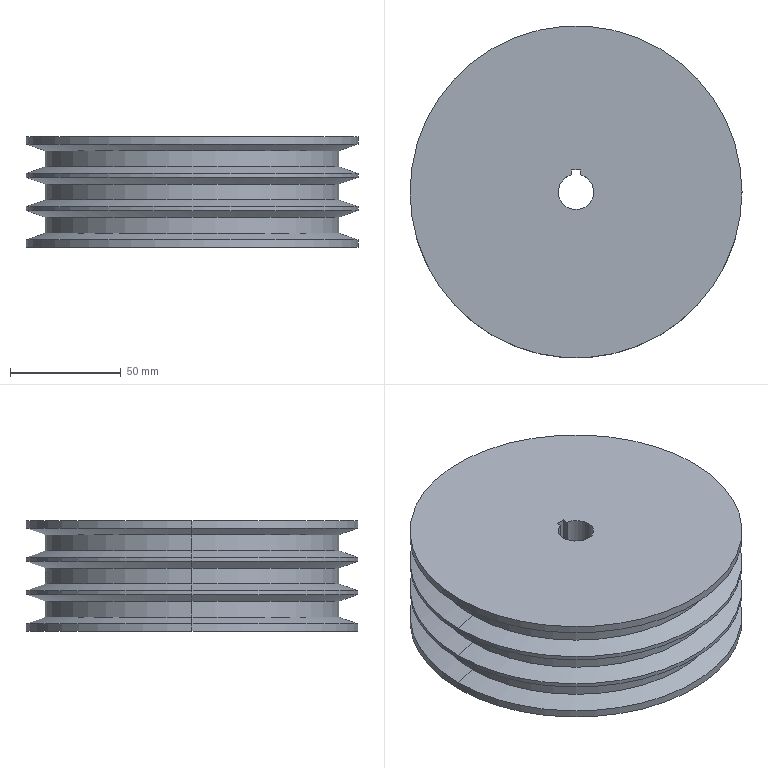Part | SolidWorks | features ICE 5, Extrusion 1, HoleWzd 1, RevCut 1 | 1 solid | 39 faces | box 150 x 150 x 50 mm | volume 752119 mm3 | cylinder 19 | cone 12 | plane 8 | commonest cylinder face diameters 150 x8 132.6 x6 16 x3 6.8 x2
STEP:
#1=CARTESIAN_POINT('',(0.,66.3,11.6));
#2=VERTEX_POINT('',#1);
#3=CARTESIAN_POINT('',(0.,66.3,18.4));
#4=VERTEX_POINT('',#3);
#5=CARTESIAN_POINT('',(0.,66.3,11.6));
#6=CARTESIAN_POINT('',(-0.2247,66.3,11.6));
#7=CARTESIAN_POINT('',(-0.4456,66.299,11.622));
#8=CARTESIAN_POINT('',(-0.8802,66.295,11.708));
#9=CARTESIAN_POINT('',(-1.096,66.291,11.774));
#10=CARTESIAN_POINT('',(-1.508,66.283,11.945));
#11=CARTESIAN_POINT('',(-1.703,66.278,12.049));
#12=CARTESIAN_POINT('',(-2.073,66.268,12.296));
#13=CARTESIAN_POINT('',(-2.248,66.262,12.439));
#14=CARTESIAN_POINT('',(-2.561,66.251,12.753));
#15=CARTESIAN_POINT('',(-2.702,66.245,12.924));
#16=CARTESIAN_POINT('',(-2.951,66.234,13.296));
#17=CARTESIAN_POINT('',(-3.056,66.23,13.494));
#18=CARTESIAN_POINT('',(-3.226,66.222,13.903));
#19=CARTESIAN_POINT('',(-3.291,66.218,14.117));
#20=CARTESIAN_POINT('',(-3.378,66.214,14.556));
#21=CARTESIAN_POINT('',(-3.4,66.213,14.777));
#22=CARTESIAN_POINT('',(-3.4,66.213,15.221));
#23=CARTESIAN_POINT('',(-3.378,66.214,15.446));
#24=CARTESIAN_POINT('',(-3.291,66.218,15.882));
#25=CARTESIAN_POINT('',(-3.227,66.221,16.094));
#26=CARTESIAN_POINT('',(-3.057,66.23,16.506));
#27=CARTESIAN_POINT('',(-2.95,66.234,16.705));
#28=CARTESIAN_POINT('',(-2.704,66.245,17.073));
#29=CARTESIAN_POINT('',(-2.563,66.251,17.245));
#30=CARTESIAN_POINT('',(-2.246,66.262,17.562));
#31=CARTESIAN_POINT('',(-2.074,66.268,17.703));
#32=CARTESIAN_POINT('',(-1.706,66.278,17.949));
#33=CARTESIAN_POINT('',(-1.507,66.283,18.056));
#34=CARTESIAN_POINT('',(-1.095,66.291,18.227));
#35=CARTESIAN_POINT('',(-0.883,66.294,18.291));
#36=CARTESIAN_POINT('',(-0.4473,66.299,18.378));
#37=CARTESIAN_POINT('',(-0.2219,66.3,18.4));
#38=CARTESIAN_POINT('',(0.,66.3,18.4));
#39=B_SPLINE_CURVE_WITH_KNOTS('',3,(#5,#6,#7,#8,#9,#10,#11,#12,#13,#14,#15,#16,#17,#18,#19,#20,#21,#22,#23,#24,#25,#26,#27,#28,#29,#30,#31,#32,#33,#34,#35,#36,#37,#38),.UNSPECIFIED.,.F.,.F.,(4,2,2,2,2,2,2,2,2,2,2,2,2,2,2,2,4),(0.,0.0006645,0.001329,0.001993,0.002658,0.003322,0.003987,0.004651,0.005316,0.00598,0.006645,0.007309,0.007974,0.008638,0.009303,0.009967,0.01063),.UNSPECIFIED.);
#40=EDGE_CURVE('',#2,#4,#39,.T.);
#41=ORIENTED_EDGE('',*,*,#40,.T.);
#42=CARTESIAN_POINT('',(0.,10.,18.4));
#43=VERTEX_POINT('',#42);
#44=CARTESIAN_POINT('',(0.,10.,18.4));
#45=DIRECTION('',(0.,-1.,0.));
#46=VECTOR('',#45,1000.);
#47=LINE('',#44,#46);
#48=EDGE_CURVE('',#4,#43,#47,.T.);
#49=ORIENTED_EDGE('',*,*,#48,.T.);
#50=CARTESIAN_POINT('',(-2.,10.,17.75));
#51=VERTEX_POINT('',#50);
#52=CARTESIAN_POINT('',(0.,10.,15.));
#53=DIRECTION('',(0.,-1.,0.));
#54=DIRECTION('',(0.,0.,-1.));
#55=AXIS2_PLACEMENT_3D('',#52,#53,#54);
#56=CIRCLE('',#55,3.4);
#57=EDGE_CURVE('',#43,#51,#56,.T.);
#58=ORIENTED_EDGE('',*,*,#57,.T.);
#59=CARTESIAN_POINT('',(-2.,10.,12.25));
#60=VERTEX_POINT('',#59);
#61=CARTESIAN_POINT('',(0.,10.,15.));
#62=DIRECTION('',(0.,-1.,0.));
#63=DIRECTION('',(0.,0.,-1.));
#64=AXIS2_PLACEMENT_3D('',#61,#62,#63);
#65=CIRCLE('',#64,3.4);
#66=EDGE_CURVE('',#51,#60,#65,.T.);
#67=ORIENTED_EDGE('',*,*,#66,.T.);
#68=CARTESIAN_POINT('',(0.,10.,11.6));
#69=VERTEX_POINT('',#68);
#70=CARTESIAN_POINT('',(0.,10.,15.));
#71=DIRECTION('',(0.,-1.,0.));
#72=DIRECTION('',(0.,0.,-1.));
#73=AXIS2_PLACEMENT_3D('',#70,#71,#72);
#74=CIRCLE('',#73,3.4);
#75=EDGE_CURVE('',#60,#69,#74,.T.);
#76=ORIENTED_EDGE('',*,*,#75,.T.);
#77=CARTESIAN_POINT('',(0.,10.,11.6));
#78=DIRECTION('',(0.,-1.,0.));
#79=VECTOR('',#78,1000.);
#80=LINE('',#77,#79);
#81=EDGE_CURVE('',#2,#69,#80,.T.);
#82=ORIENTED_EDGE('',*,*,#81,.F.);
#83=EDGE_LOOP('',(#41,#49,#58,#67,#76,#82));
#84=FACE_OUTER_BOUND('',#83,.T.);
#85=CARTESIAN_POINT('',(0.,10.,15.));
#86=DIRECTION('',(0.,-1.,0.));
#87=DIRECTION('',(0.,0.,-1.));
#88=AXIS2_PLACEMENT_3D('',#85,#86,#87);
#89=CYLINDRICAL_SURFACE('',#88,3.4);
#90=ADVANCED_FACE('',(#84),#89,.F.);
#91=CARTESIAN_POINT('',(66.3,0.,26.396));
#92=VERTEX_POINT('',#91);
#93=CARTESIAN_POINT('',(-66.3,0.,26.396));
#94=VERTEX_POINT('',#93);
#95=CARTESIAN_POINT('',(0.,0.,26.396));
#96=DIRECTION('',(0.,0.,1.));
#97=DIRECTION('',(1.,0.,0.));
#98=AXIS2_PLACEMENT_3D('',#95,#96,#97);
#99=CIRCLE('',#98,66.3);
#100=EDGE_CURVE('',#92,#94,#99,.T.);
#101=ORIENTED_EDGE('',*,*,#100,.F.);
#102=CARTESIAN_POINT('',(75.,0.,23.4));
#103=VERTEX_POINT('',#102);
#104=CARTESIAN_POINT('',(66.3,0.,26.396));
#105=DIRECTION('',(0.9455,0.,-0.3256));
#106=VECTOR('',#105,1000.);
#107=LINE('',#104,#106);
#108=EDGE_CURVE('',#92,#103,#107,.T.);
#109=ORIENTED_EDGE('',*,*,#108,.T.);
#110=CARTESIAN_POINT('',(-75.,0.,23.4));
#111=VERTEX_POINT('',#110);
#112=CARTESIAN_POINT('',(0.,0.,23.4));
#113=DIRECTION('',(0.,0.,1.));
#114=DIRECTION('',(1.,0.,0.));
#115=AXIS2_PLACEMENT_3D('',#112,#113,#114);
#116=CIRCLE('',#115,75.);
#117=EDGE_CURVE('',#103,#111,#116,.T.);
#118=ORIENTED_EDGE('',*,*,#117,.T.);
#119=CARTESIAN_POINT('',(-66.3,0.,26.396));
#120=DIRECTION('',(-0.9455,0.,-0.3256));
#121=VECTOR('',#120,1000.);
#122=LINE('',#119,#121);
#123=EDGE_CURVE('',#94,#111,#122,.T.);
#124=ORIENTED_EDGE('',*,*,#123,.F.);
#125=EDGE_LOOP('',(#101,#109,#118,#124));
#126=FACE_OUTER_BOUND('',#125,.T.);
#127=CARTESIAN_POINT('',(0.,0.,26.396));
#128=DIRECTION('',(0.,0.,-1.));
#129=DIRECTION('',(-1.,0.,0.));
#130=AXIS2_PLACEMENT_3D('',#127,#128,#129);
#131=CONICAL_SURFACE('',#130,66.3,1.239);
#132=ADVANCED_FACE('',(#126),#131,.T.);
#133=ORIENTED_EDGE('',*,*,#100,.T.);
#134=CARTESIAN_POINT('',(-66.3,0.,33.604));
#135=VERTEX_POINT('',#134);
#136=CARTESIAN_POINT('',(-66.3,0.,0.));
#137=DIRECTION('',(0.,0.,1.));
#138=VECTOR('',#137,1000.);
#139=LINE('',#136,#138);
#140=EDGE_CURVE('',#94,#135,#139,.T.);
#141=ORIENTED_EDGE('',*,*,#140,.T.);
#142=CARTESIAN_POINT('',(66.3,0.,33.604));
#143=VERTEX_POINT('',#142);
#144=CARTESIAN_POINT('',(0.,0.,33.604));
#145=DIRECTION('',(0.,0.,1.));
#146=DIRECTION('',(1.,0.,0.));
#147=AXIS2_PLACEMENT_3D('',#144,#145,#146);
#148=CIRCLE('',#147,66.3);
#149=EDGE_CURVE('',#143,#135,#148,.T.);
#150=ORIENTED_EDGE('',*,*,#149,.F.);
#151=CARTESIAN_POINT('',(66.3,0.,0.));
#152=DIRECTION('',(0.,0.,1.));
#153=VECTOR('',#152,1000.);
#154=LINE('',#151,#153);
#155=EDGE_CURVE('',#92,#143,#154,.T.);
#156=ORIENTED_EDGE('',*,*,#155,.F.);
#157=EDGE_LOOP('',(#133,#141,#150,#156));
#158=FACE_OUTER_BOUND('',#157,.T.);
#159=CARTESIAN_POINT('',(0.,0.,0.));
#160=DIRECTION('',(0.,0.,1.));
#161=DIRECTION('',(1.,0.,0.));
#162=AXIS2_PLACEMENT_3D('',#159,#160,#161);
#163=CYLINDRICAL_SURFACE('',#162,66.3);
#164=ADVANCED_FACE('',(#158),#163,.T.);
#165=ORIENTED_EDGE('',*,*,#149,.T.);
#166=CARTESIAN_POINT('',(-75.,0.,36.6));
#167=VERTEX_POINT('',#166);
#168=CARTESIAN_POINT('',(-75.,0.,36.6));
#169=DIRECTION('',(-0.9455,0.,0.3256));
#170=VECTOR('',#169,1000.);
#171=LINE('',#168,#170);
#172=EDGE_CURVE('',#135,#167,#171,.T.);
#173=ORIENTED_EDGE('',*,*,#172,.T.);
#174=CARTESIAN_POINT('',(75.,0.,36.6));
#175=VERTEX_POINT('',#174);
#176=CARTESIAN_POINT('',(0.,0.,36.6));
#177=DIRECTION('',(0.,0.,1.));
#178=DIRECTION('',(1.,0.,0.));
#179=AXIS2_PLACEMENT_3D('',#176,#177,#178);
#180=CIRCLE('',#179,75.);
#181=EDGE_CURVE('',#175,#167,#180,.T.);
#182=ORIENTED_EDGE('',*,*,#181,.F.);
#183=CARTESIAN_POINT('',(75.,0.,36.6));
#184=DIRECTION('',(0.9455,0.,0.3256));
#185=VECTOR('',#184,1000.);
#186=LINE('',#183,#185);
#187=EDGE_CURVE('',#143,#175,#186,.T.);
#188=ORIENTED_EDGE('',*,*,#187,.F.);
#189=EDGE_LOOP('',(#165,#173,#182,#188));
#190=FACE_OUTER_BOUND('',#189,.T.);
#191=CARTESIAN_POINT('',(0.,0.,36.6));
#192=DIRECTION('',(0.,0.,1.));
#193=DIRECTION('',(1.,0.,0.));
#194=AXIS2_PLACEMENT_3D('',#191,#192,#193);
#195=CONICAL_SURFACE('',#194,75.,1.239);
#196=ADVANCED_FACE('',(#190),#195,.T.);
#197=ORIENTED_EDGE('',*,*,#117,.F.);
#198=CARTESIAN_POINT('',(75.,0.,21.6));
#199=VERTEX_POINT('',#198);
#200=CARTESIAN_POINT('',(75.,0.,40.));
#201=DIRECTION('',(0.,0.,-1.));
#202=VECTOR('',#201,1000.);
#203=LINE('',#200,#202);
#204=EDGE_CURVE('',#103,#199,#203,.T.);
#205=ORIENTED_EDGE('',*,*,#204,.T.);
#206=CARTESIAN_POINT('',(-75.,0.,21.6));
#207=VERTEX_POINT('',#206);
#208=CARTESIAN_POINT('',(0.,0.,21.6));
#209=DIRECTION('',(0.,0.,1.));
#210=DIRECTION('',(1.,0.,0.));
#211=AXIS2_PLACEMENT_3D('',#208,#209,#210);
#212=CIRCLE('',#211,75.);
#213=EDGE_CURVE('',#199,#207,#212,.T.);
#214=ORIENTED_EDGE('',*,*,#213,.T.);
#215=CARTESIAN_POINT('',(-75.,0.,40.));
#216=DIRECTION('',(0.,0.,-1.));
#217=VECTOR('',#216,1000.);
#218=LINE('',#215,#217);
#219=EDGE_CURVE('',#111,#207,#218,.T.);
#220=ORIENTED_EDGE('',*,*,#219,.F.);
#221=EDGE_LOOP('',(#197,#205,#214,#220));
#222=FACE_OUTER_BOUND('',#221,.T.);
#223=CARTESIAN_POINT('',(0.,0.,40.));
#224=DIRECTION('',(0.,0.,-1.));
#225=DIRECTION('',(-1.,0.,0.));
#226=AXIS2_PLACEMENT_3D('',#223,#224,#225);
#227=CYLINDRICAL_SURFACE('',#226,75.);
#228=ADVANCED_FACE('',(#222),#227,.T.);
#229=CARTESIAN_POINT('',(66.3,0.,11.396));
#230=VERTEX_POINT('',#229);
#231=CARTESIAN_POINT('',(-66.3,0.,11.396));
#232=VERTEX_POINT('',#231);
#233=CARTESIAN_POINT('',(0.,0.,11.396));
#234=DIRECTION('',(0.,0.,1.));
#235=DIRECTION('',(1.,0.,0.));
#236=AXIS2_PLACEMENT_3D('',#233,#234,#235);
#237=CIRCLE('',#236,66.3);
#238=EDGE_CURVE('',#230,#232,#237,.T.);
#239=ORIENTED_EDGE('',*,*,#238,.F.);
#240=CARTESIAN_POINT('',(75.,0.,8.4));
#241=VERTEX_POINT('',#240);
#242=CARTESIAN_POINT('',(66.3,0.,11.396));
#243=DIRECTION('',(0.9455,0.,-0.3256));
#244=VECTOR('',#243,1000.);
#245=LINE('',#242,#244);
#246=EDGE_CURVE('',#230,#241,#245,.T.);
#247=ORIENTED_EDGE('',*,*,#246,.T.);
#248=CARTESIAN_POINT('',(-75.,0.,8.4));
#249=VERTEX_POINT('',#248);
#250=CARTESIAN_POINT('',(0.,0.,8.4));
#251=DIRECTION('',(0.,0.,1.));
#252=DIRECTION('',(1.,0.,0.));
#253=AXIS2_PLACEMENT_3D('',#250,#251,#252);
#254=CIRCLE('',#253,75.);
#255=EDGE_CURVE('',#241,#249,#254,.T.);
#256=ORIENTED_EDGE('',*,*,#255,.T.);
#257=CARTESIAN_POINT('',(-66.3,0.,11.396));
#258=DIRECTION('',(-0.9455,0.,-0.3256));
#259=VECTOR('',#258,1000.);
#260=LINE('',#257,#259);
#261=EDGE_CURVE('',#232,#249,#260,.T.);
#262=ORIENTED_EDGE('',*,*,#261,.F.);
#263=EDGE_LOOP('',(#239,#247,#256,#262));
#264=FACE_OUTER_BOUND('',#263,.T.);
#265=CARTESIAN_POINT('',(0.,0.,11.396));
#266=DIRECTION('',(0.,0.,-1.));
#267=DIRECTION('',(-1.,0.,0.));
#268=AXIS2_PLACEMENT_3D('',#265,#266,#267);
#269=CONICAL_SURFACE('',#268,66.3,1.239);
#270=ADVANCED_FACE('',(#264),#269,.T.);
#271=ORIENTED_EDGE('',*,*,#40,.F.);
#272=CARTESIAN_POINT('',(0.,66.3,18.4));
#273=CARTESIAN_POINT('',(0.2219,66.3,18.4));
#274=CARTESIAN_POINT('',(0.4424,66.299,18.378));
#275=CARTESIAN_POINT('',(0.8807,66.295,18.292));
#276=CARTESIAN_POINT('',(1.096,66.291,18.226));
#277=CARTESIAN_POINT('',(1.505,66.283,18.057));
#278=CARTESIAN_POINT('',(1.702,66.278,17.952));
#279=CARTESIAN_POINT('',(2.074,66.268,17.703));
#280=CARTESIAN_POINT('',(2.246,66.262,17.562));
#281=CARTESIAN_POINT('',(2.559,66.251,17.249));
#282=CARTESIAN_POINT('',(2.703,66.245,17.075));
#283=CARTESIAN_POINT('',(2.95,66.234,16.705));
#284=CARTESIAN_POINT('',(3.055,66.23,16.51));
#285=CARTESIAN_POINT('',(3.225,66.222,16.099));
#286=CARTESIAN_POINT('',(3.291,66.218,15.882));
#287=CARTESIAN_POINT('',(3.378,66.214,15.448));
#288=CARTESIAN_POINT('',(3.4,66.213,15.227));
#289=CARTESIAN_POINT('',(3.4,66.213,14.779));
#290=CARTESIAN_POINT('',(3.378,66.214,14.557));
#291=CARTESIAN_POINT('',(3.292,66.218,14.122));
#292=CARTESIAN_POINT('',(3.227,66.221,13.907));
#293=CARTESIAN_POINT('',(3.057,66.23,13.494));
#294=CARTESIAN_POINT('',(2.952,66.234,13.299));
#295=CARTESIAN_POINT('',(2.706,66.245,12.93));
#296=CARTESIAN_POINT('',(2.563,66.251,12.755));
#297=CARTESIAN_POINT('',(2.249,66.262,12.441));
#298=CARTESIAN_POINT('',(2.078,66.268,12.3));
#299=CARTESIAN_POINT('',(1.707,66.278,12.051));
#300=CARTESIAN_POINT('',(1.509,66.283,11.945));
#301=CARTESIAN_POINT('',(0.8956,66.295,11.69));
#302=CARTESIAN_POINT('',(0.4493,66.3,11.6));
#303=CARTESIAN_POINT('',(0.,66.3,11.6));
#304=B_SPLINE_CURVE_WITH_KNOTS('',3,(#272,#273,#274,#275,#276,#277,#278,#279,#280,#281,#282,#283,#284,#285,#286,#287,#288,#289,#290,#291,#292,#293,#294,#295,#296,#297,#298,#299,#300,#301,#302,#303),.UNSPECIFIED.,.F.,.F.,(4,2,2,2,2,2,2,2,2,2,2,2,2,2,2,4),(0.01063,0.0113,0.01196,0.01262,0.01329,0.01395,0.01462,0.01528,0.01595,0.01661,0.01727,0.01794,0.0186,0.01927,0.01993,0.02126),.UNSPECIFIED.);
#305=EDGE_CURVE('',#4,#2,#304,.T.);
#306=ORIENTED_EDGE('',*,*,#305,.F.);
#307=EDGE_LOOP('',(#271,#306));
#308=FACE_BOUND('',#307,.T.);
#309=ORIENTED_EDGE('',*,*,#238,.T.);
#310=CARTESIAN_POINT('',(-66.3,0.,18.604));
#311=VERTEX_POINT('',#310);
#312=CARTESIAN_POINT('',(-66.3,0.,0.));
#313=DIRECTION('',(0.,0.,1.));
#314=VECTOR('',#313,1000.);
#315=LINE('',#312,#314);
#316=EDGE_CURVE('',#232,#311,#315,.T.);
#317=ORIENTED_EDGE('',*,*,#316,.T.);
#318=CARTESIAN_POINT('',(66.3,0.,18.604));
#319=VERTEX_POINT('',#318);
#320=CARTESIAN_POINT('',(0.,0.,18.604));
#321=DIRECTION('',(0.,0.,1.));
#322=DIRECTION('',(1.,0.,0.));
#323=AXIS2_PLACEMENT_3D('',#320,#321,#322);
#324=CIRCLE('',#323,66.3);
#325=EDGE_CURVE('',#319,#311,#324,.T.);
#326=ORIENTED_EDGE('',*,*,#325,.F.);
#327=CARTESIAN_POINT('',(66.3,0.,0.));
#328=DIRECTION('',(0.,0.,1.));
#329=VECTOR('',#328,1000.);
#330=LINE('',#327,#329);
#331=EDGE_CURVE('',#230,#319,#330,.T.);
#332=ORIENTED_EDGE('',*,*,#331,.F.);
#333=EDGE_LOOP('',(#309,#317,#326,#332));
#334=FACE_OUTER_BOUND('',#333,.T.);
#335=CARTESIAN_POINT('',(0.,0.,0.));
#336=DIRECTION('',(0.,0.,1.));
#337=DIRECTION('',(1.,0.,0.));
#338=AXIS2_PLACEMENT_3D('',#335,#336,#337);
#339=CYLINDRICAL_SURFACE('',#338,66.3);
#340=ADVANCED_FACE('',(#308,#334),#339,.T.);
#341=ORIENTED_EDGE('',*,*,#325,.T.);
#342=CARTESIAN_POINT('',(-75.,0.,21.6));
#343=DIRECTION('',(-0.9455,0.,0.3256));
#344=VECTOR('',#343,1000.);
#345=LINE('',#342,#344);
#346=EDGE_CURVE('',#311,#207,#345,.T.);
#347=ORIENTED_EDGE('',*,*,#346,.T.);
#348=ORIENTED_EDGE('',*,*,#213,.F.);
#349=CARTESIAN_POINT('',(75.,0.,21.6));
#350=DIRECTION('',(0.9455,0.,0.3256));
#351=VECTOR('',#350,1000.);
#352=LINE('',#349,#351);
#353=EDGE_CURVE('',#319,#199,#352,.T.);
#354=ORIENTED_EDGE('',*,*,#353,.F.);
#355=EDGE_LOOP('',(#341,#347,#348,#354));
#356=FACE_OUTER_BOUND('',#355,.T.);
#357=CARTESIAN_POINT('',(0.,0.,21.6));
#358=DIRECTION('',(0.,0.,1.));
#359=DIRECTION('',(1.,0.,0.));
#360=AXIS2_PLACEMENT_3D('',#357,#358,#359);
#361=CONICAL_SURFACE('',#360,75.,1.239);
#362=ADVANCED_FACE('',(#356),#361,.T.);
#363=ORIENTED_EDGE('',*,*,#255,.F.);
#364=CARTESIAN_POINT('',(75.,0.,6.6));
#365=VERTEX_POINT('',#364);
#366=CARTESIAN_POINT('',(75.,0.,40.));
#367=DIRECTION('',(0.,0.,-1.));
#368=VECTOR('',#367,1000.);
#369=LINE('',#366,#368);
#370=EDGE_CURVE('',#241,#365,#369,.T.);
#371=ORIENTED_EDGE('',*,*,#370,.T.);
#372=CARTESIAN_POINT('',(-75.,0.,6.6));
#373=VERTEX_POINT('',#372);
#374=CARTESIAN_POINT('',(0.,0.,6.6));
#375=DIRECTION('',(0.,0.,1.));
#376=DIRECTION('',(1.,0.,0.));
#377=AXIS2_PLACEMENT_3D('',#374,#375,#376);
#378=CIRCLE('',#377,75.);
#379=EDGE_CURVE('',#365,#373,#378,.T.);
#380=ORIENTED_EDGE('',*,*,#379,.T.);
#381=CARTESIAN_POINT('',(-75.,0.,40.));
#382=DIRECTION('',(0.,0.,-1.));
#383=VECTOR('',#382,1000.);
#384=LINE('',#381,#383);
#385=EDGE_CURVE('',#249,#373,#384,.T.);
#386=ORIENTED_EDGE('',*,*,#385,.F.);
#387=EDGE_LOOP('',(#363,#371,#380,#386));
#388=FACE_OUTER_BOUND('',#387,.T.);
#389=CARTESIAN_POINT('',(0.,0.,40.));
#390=DIRECTION('',(0.,0.,-1.));
#391=DIRECTION('',(-1.,0.,0.));
#392=AXIS2_PLACEMENT_3D('',#389,#390,#391);
#393=CYLINDRICAL_SURFACE('',#392,75.);
#394=ADVANCED_FACE('',(#388),#393,.T.);
#395=CARTESIAN_POINT('',(66.3,0.,-3.604));
#396=VERTEX_POINT('',#395);
#397=CARTESIAN_POINT('',(-66.3,0.,-3.604));
#398=VERTEX_POINT('',#397);
#399=CARTESIAN_POINT('',(0.,0.,-3.604));
#400=DIRECTION('',(0.,0.,1.));
#401=DIRECTION('',(1.,0.,0.));
#402=AXIS2_PLACEMENT_3D('',#399,#400,#401);
#403=CIRCLE('',#402,66.3);
#404=EDGE_CURVE('',#396,#398,#403,.T.);
#405=ORIENTED_EDGE('',*,*,#404,.F.);
#406=CARTESIAN_POINT('',(75.,0.,-6.6));
#407=VERTEX_POINT('',#406);
#408=CARTESIAN_POINT('',(66.3,0.,-3.604));
#409=DIRECTION('',(0.9455,0.,-0.3256));
#410=VECTOR('',#409,1000.);
#411=LINE('',#408,#410);
#412=EDGE_CURVE('',#396,#407,#411,.T.);
#413=ORIENTED_EDGE('',*,*,#412,.T.);
#414=CARTESIAN_POINT('',(-75.,0.,-6.6));
#415=VERTEX_POINT('',#414);
#416=CARTESIAN_POINT('',(0.,0.,-6.6));
#417=DIRECTION('',(0.,0.,1.));
#418=DIRECTION('',(1.,0.,0.));
#419=AXIS2_PLACEMENT_3D('',#416,#417,#418);
#420=CIRCLE('',#419,75.);
#421=EDGE_CURVE('',#407,#415,#420,.T.);
#422=ORIENTED_EDGE('',*,*,#421,.T.);
#423=CARTESIAN_POINT('',(-66.3,0.,-3.604));
#424=DIRECTION('',(-0.9455,0.,-0.3256));
#425=VECTOR('',#424,1000.);
#426=LINE('',#423,#425);
#427=EDGE_CURVE('',#398,#415,#426,.T.);
#428=ORIENTED_EDGE('',*,*,#427,.F.);
#429=EDGE_LOOP('',(#405,#413,#422,#428));
#430=FACE_OUTER_BOUND('',#429,.T.);
#431=CARTESIAN_POINT('',(0.,0.,-3.604));
#432=DIRECTION('',(0.,0.,-1.));
#433=DIRECTION('',(-1.,0.,0.));
#434=AXIS2_PLACEMENT_3D('',#431,#432,#433);
#435=CONICAL_SURFACE('',#434,66.3,1.239);
#436=ADVANCED_FACE('',(#430),#435,.T.);
#437=ORIENTED_EDGE('',*,*,#404,.T.);
#438=CARTESIAN_POINT('',(-66.3,0.,3.604));
#439=VERTEX_POINT('',#438);
#440=CARTESIAN_POINT('',(-66.3,0.,0.));
#441=DIRECTION('',(0.,0.,1.));
#442=VECTOR('',#441,1000.);
#443=LINE('',#440,#442);
#444=EDGE_CURVE('',#398,#439,#443,.T.);
#445=ORIENTED_EDGE('',*,*,#444,.T.);
#446=CARTESIAN_POINT('',(66.3,0.,3.604));
#447=VERTEX_POINT('',#446);
#448=CARTESIAN_POINT('',(0.,0.,3.604));
#449=DIRECTION('',(0.,0.,1.));
#450=DIRECTION('',(1.,0.,0.));
#451=AXIS2_PLACEMENT_3D('',#448,#449,#450);
#452=CIRCLE('',#451,66.3);
#453=EDGE_CURVE('',#447,#439,#452,.T.);
#454=ORIENTED_EDGE('',*,*,#453,.F.);
#455=CARTESIAN_POINT('',(66.3,0.,0.));
#456=DIRECTION('',(0.,0.,1.));
#457=VECTOR('',#456,1000.);
#458=LINE('',#455,#457);
#459=EDGE_CURVE('',#396,#447,#458,.T.);
#460=ORIENTED_EDGE('',*,*,#459,.F.);
#461=EDGE_LOOP('',(#437,#445,#454,#460));
#462=FACE_OUTER_BOUND('',#461,.T.);
#463=CARTESIAN_POINT('',(0.,0.,0.));
#464=DIRECTION('',(0.,0.,1.));
#465=DIRECTION('',(1.,0.,0.));
#466=AXIS2_PLACEMENT_3D('',#463,#464,#465);
#467=CYLINDRICAL_SURFACE('',#466,66.3);
#468=ADVANCED_FACE('',(#462),#467,.T.);
#469=ORIENTED_EDGE('',*,*,#453,.T.);
#470=CARTESIAN_POINT('',(-75.,0.,6.6));
#471=DIRECTION('',(-0.9455,0.,0.3256));
#472=VECTOR('',#471,1000.);
#473=LINE('',#470,#472);
#474=EDGE_CURVE('',#439,#373,#473,.T.);
#475=ORIENTED_EDGE('',*,*,#474,.T.);
#476=ORIENTED_EDGE('',*,*,#379,.F.);
#477=CARTESIAN_POINT('',(75.,0.,6.6));
#478=DIRECTION('',(0.9455,0.,0.3256));
#479=VECTOR('',#478,1000.);
#480=LINE('',#477,#479);
#481=EDGE_CURVE('',#447,#365,#480,.T.);
#482=ORIENTED_EDGE('',*,*,#481,.F.);
#483=EDGE_LOOP('',(#469,#475,#476,#482));
#484=FACE_OUTER_BOUND('',#483,.T.);
#485=CARTESIAN_POINT('',(0.,0.,6.6));
#486=DIRECTION('',(0.,0.,1.));
#487=DIRECTION('',(1.,0.,0.));
#488=AXIS2_PLACEMENT_3D('',#485,#486,#487);
#489=CONICAL_SURFACE('',#488,75.,1.239);
#490=ADVANCED_FACE('',(#484),#489,.T.);
#491=CARTESIAN_POINT('',(75.,0.,40.));
#492=VERTEX_POINT('',#491);
#493=CARTESIAN_POINT('',(-75.,0.,40.));
#494=VERTEX_POINT('',#493);
#495=CARTESIAN_POINT('',(0.,0.,40.));
#496=DIRECTION('',(0.,0.,1.));
#497=DIRECTION('',(1.,0.,0.));
#498=AXIS2_PLACEMENT_3D('',#495,#496,#497);
#499=CIRCLE('',#498,75.);
#500=EDGE_CURVE('',#492,#494,#499,.T.);
#501=ORIENTED_EDGE('',*,*,#500,.F.);
#502=CARTESIAN_POINT('',(75.,0.,40.));
#503=DIRECTION('',(0.,0.,-1.));
#504=VECTOR('',#503,1000.);
#505=LINE('',#502,#504);
#506=EDGE_CURVE('',#492,#175,#505,.T.);
#507=ORIENTED_EDGE('',*,*,#506,.T.);
#508=ORIENTED_EDGE('',*,*,#181,.T.);
#509=CARTESIAN_POINT('',(-75.,0.,40.));
#510=DIRECTION('',(0.,0.,-1.));
#511=VECTOR('',#510,1000.);
#512=LINE('',#509,#511);
#513=EDGE_CURVE('',#494,#167,#512,.T.);
#514=ORIENTED_EDGE('',*,*,#513,.F.);
#515=EDGE_LOOP('',(#501,#507,#508,#514));
#516=FACE_OUTER_BOUND('',#515,.T.);
#517=CARTESIAN_POINT('',(0.,0.,40.));
#518=DIRECTION('',(0.,0.,-1.));
#519=DIRECTION('',(-1.,0.,0.));
#520=AXIS2_PLACEMENT_3D('',#517,#518,#519);
#521=CYLINDRICAL_SURFACE('',#520,75.);
#522=ADVANCED_FACE('',(#516),#521,.T.);
#523=CARTESIAN_POINT('',(-8.,0.,-10.));
#524=VERTEX_POINT('',#523);
#525=CARTESIAN_POINT('',(8.,0.,-10.));
#526=VERTEX_POINT('',#525);
#527=CARTESIAN_POINT('',(0.,0.,-10.));
#528=DIRECTION('',(0.,0.,1.));
#529=DIRECTION('',(-1.,0.,0.));
#530=AXIS2_PLACEMENT_3D('',#527,#528,#529);
#531=CIRCLE('',#530,8.);
#532=EDGE_CURVE('',#524,#526,#531,.T.);
#533=ORIENTED_EDGE('',*,*,#532,.F.);
#534=CARTESIAN_POINT('',(-8.,0.,40.));
#535=VERTEX_POINT('',#534);
#536=CARTESIAN_POINT('',(-8.,0.,-110.));
#537=DIRECTION('',(0.,0.,1.));
#538=VECTOR('',#537,1000.);
#539=LINE('',#536,#538);
#540=EDGE_CURVE('',#524,#535,#539,.T.);
#541=ORIENTED_EDGE('',*,*,#540,.T.);
#542=CARTESIAN_POINT('',(8.,0.,40.));
#543=VERTEX_POINT('',#542);
#544=CARTESIAN_POINT('',(0.,0.,40.));
#545=DIRECTION('',(0.,0.,1.));
#546=DIRECTION('',(1.,0.,0.));
#547=AXIS2_PLACEMENT_3D('',#544,#545,#546);
#548=CIRCLE('',#547,8.);
#549=EDGE_CURVE('',#535,#543,#548,.T.);
#550=ORIENTED_EDGE('',*,*,#549,.T.);
#551=CARTESIAN_POINT('',(8.,0.,-110.));
#552=DIRECTION('',(0.,0.,1.));
#553=VECTOR('',#552,1000.);
#554=LINE('',#551,#553);
#555=EDGE_CURVE('',#526,#543,#554,.T.);
#556=ORIENTED_EDGE('',*,*,#555,.F.);
#557=EDGE_LOOP('',(#533,#541,#550,#556));
#558=FACE_OUTER_BOUND('',#557,.T.);
#559=CARTESIAN_POINT('',(0.,0.,-110.));
#560=DIRECTION('',(0.,0.,1.));
#561=DIRECTION('',(1.,0.,0.));
#562=AXIS2_PLACEMENT_3D('',#559,#560,#561);
#563=CYLINDRICAL_SURFACE('',#562,8.);
#564=ADVANCED_FACE('',(#558),#563,.F.);
#565=CARTESIAN_POINT('',(2.,7.746,-10.));
#566=VERTEX_POINT('',#565);
#567=CARTESIAN_POINT('',(0.,0.,-10.));
#568=DIRECTION('',(0.,0.,1.));
#569=DIRECTION('',(-1.,0.,0.));
#570=AXIS2_PLACEMENT_3D('',#567,#568,#569);
#571=CIRCLE('',#570,8.);
#572=EDGE_CURVE('',#526,#566,#571,.T.);
#573=ORIENTED_EDGE('',*,*,#572,.F.);
#574=ORIENTED_EDGE('',*,*,#555,.T.);
#575=CARTESIAN_POINT('',(2.,7.746,40.));
#576=VERTEX_POINT('',#575);
#577=CARTESIAN_POINT('',(0.,0.,40.));
#578=DIRECTION('',(0.,0.,1.));
#579=DIRECTION('',(1.,0.,0.));
#580=AXIS2_PLACEMENT_3D('',#577,#578,#579);
#581=CIRCLE('',#580,8.);
#582=EDGE_CURVE('',#543,#576,#581,.T.);
#583=ORIENTED_EDGE('',*,*,#582,.T.);
#584=CARTESIAN_POINT('',(2.,7.746,-110.));
#585=DIRECTION('',(0.,0.,-1.));
#586=VECTOR('',#585,1000.);
#587=LINE('',#584,#586);
#588=EDGE_CURVE('',#576,#566,#587,.T.);
#589=ORIENTED_EDGE('',*,*,#588,.T.);
#590=EDGE_LOOP('',(#573,#574,#583,#589));
#591=FACE_OUTER_BOUND('',#590,.T.);
#592=CARTESIAN_POINT('',(0.,0.,-110.));
#593=DIRECTION('',(0.,0.,1.));
#594=DIRECTION('',(1.,0.,0.));
#595=AXIS2_PLACEMENT_3D('',#592,#593,#594);
#596=CYLINDRICAL_SURFACE('',#595,8.);
#597=ADVANCED_FACE('',(#591),#596,.F.);
#598=ORIENTED_EDGE('',*,*,#421,.F.);
#599=CARTESIAN_POINT('',(75.,0.,-10.));
#600=VERTEX_POINT('',#599);
#601=CARTESIAN_POINT('',(75.,0.,40.));
#602=DIRECTION('',(0.,0.,-1.));
#603=VECTOR('',#602,1000.);
#604=LINE('',#601,#603);
#605=EDGE_CURVE('',#407,#600,#604,.T.);
#606=ORIENTED_EDGE('',*,*,#605,.T.);
#607=CARTESIAN_POINT('',(-75.,0.,-10.));
#608=VERTEX_POINT('',#607);
#609=CARTESIAN_POINT('',(0.,0.,-10.));
#610=DIRECTION('',(0.,0.,-1.));
#611=DIRECTION('',(-1.,0.,0.));
#612=AXIS2_PLACEMENT_3D('',#609,#610,#611);
#613=CIRCLE('',#612,75.);
#614=EDGE_CURVE('',#608,#600,#613,.T.);
#615=ORIENTED_EDGE('',*,*,#614,.F.);
#616=CARTESIAN_POINT('',(-75.,0.,40.));
#617=DIRECTION('',(0.,0.,-1.));
#618=VECTOR('',#617,1000.);
#619=LINE('',#616,#618);
#620=EDGE_CURVE('',#415,#608,#619,.T.);
#621=ORIENTED_EDGE('',*,*,#620,.F.);
#622=EDGE_LOOP('',(#598,#606,#615,#621));
#623=FACE_OUTER_BOUND('',#622,.T.);
#624=CARTESIAN_POINT('',(0.,0.,40.));
#625=DIRECTION('',(0.,0.,-1.));
#626=DIRECTION('',(-1.,0.,0.));
#627=AXIS2_PLACEMENT_3D('',#624,#625,#626);
#628=CYLINDRICAL_SURFACE('',#627,75.);
#629=ADVANCED_FACE('',(#623),#628,.T.);
#630=CARTESIAN_POINT('',(-2.,10.,40.));
#631=VERTEX_POINT('',#630);
#632=CARTESIAN_POINT('',(-2.,10.,490.));
#633=DIRECTION('',(0.,0.,-1.));
#634=VECTOR('',#633,1000.);
#635=LINE('',#632,#634);
#636=EDGE_CURVE('',#631,#51,#635,.T.);
#637=ORIENTED_EDGE('',*,*,#636,.T.);
#638=ORIENTED_EDGE('',*,*,#57,.F.);
#639=CARTESIAN_POINT('',(2.,10.,17.75));
#640=VERTEX_POINT('',#639);
#641=CARTESIAN_POINT('',(0.,10.,15.));
#642=DIRECTION('',(0.,-1.,0.));
#643=DIRECTION('',(0.,0.,-1.));
#644=AXIS2_PLACEMENT_3D('',#641,#642,#643);
#645=CIRCLE('',#644,3.4);
#646=EDGE_CURVE('',#640,#43,#645,.T.);
#647=ORIENTED_EDGE('',*,*,#646,.F.);
#648=CARTESIAN_POINT('',(2.,10.,40.));
#649=VERTEX_POINT('',#648);
#650=CARTESIAN_POINT('',(2.,10.,490.));
#651=DIRECTION('',(0.,0.,-1.));
#652=VECTOR('',#651,1000.);
#653=LINE('',#650,#652);
#654=EDGE_CURVE('',#649,#640,#653,.T.);
#655=ORIENTED_EDGE('',*,*,#654,.F.);
#656=CARTESIAN_POINT('',(0.,10.,40.));
#657=DIRECTION('',(-1.,0.,0.));
#658=VECTOR('',#657,1000.);
#659=LINE('',#656,#658);
#660=EDGE_CURVE('',#649,#631,#659,.T.);
#661=ORIENTED_EDGE('',*,*,#660,.T.);
#662=EDGE_LOOP('',(#637,#638,#647,#655,#661));
#663=FACE_OUTER_BOUND('',#662,.T.);
#664=CARTESIAN_POINT('',(2.,10.,490.));
#665=DIRECTION('',(0.,1.,0.));
#666=DIRECTION('',(-1.,0.,0.));
#667=AXIS2_PLACEMENT_3D('',#664,#665,#666);
#668=PLANE('',#667);
#669=ADVANCED_FACE('',(#663),#668,.F.);
#670=ORIENTED_EDGE('',*,*,#605,.F.);
#671=CARTESIAN_POINT('',(0.,0.,-6.6));
#672=DIRECTION('',(0.,0.,1.));
#673=DIRECTION('',(1.,0.,0.));
#674=AXIS2_PLACEMENT_3D('',#671,#672,#673);
#675=CIRCLE('',#674,75.);
#676=EDGE_CURVE('',#415,#407,#675,.T.);
#677=ORIENTED_EDGE('',*,*,#676,.F.);
#678=ORIENTED_EDGE('',*,*,#620,.T.);
#679=CARTESIAN_POINT('',(0.,0.,-10.));
#680=DIRECTION('',(0.,0.,-1.));
#681=DIRECTION('',(-1.,0.,0.));
#682=AXIS2_PLACEMENT_3D('',#679,#680,#681);
#683=CIRCLE('',#682,75.);
#684=EDGE_CURVE('',#600,#608,#683,.T.);
#685=ORIENTED_EDGE('',*,*,#684,.F.);
#686=EDGE_LOOP('',(#670,#677,#678,#685));
#687=FACE_OUTER_BOUND('',#686,.T.);
#688=CARTESIAN_POINT('',(0.,0.,40.));
#689=DIRECTION('',(0.,0.,-1.));
#690=DIRECTION('',(-1.,0.,0.));
#691=AXIS2_PLACEMENT_3D('',#688,#689,#690);
#692=CYLINDRICAL_SURFACE('',#691,75.);
#693=ADVANCED_FACE('',(#687),#692,.T.);
#694=ORIENTED_EDGE('',*,*,#540,.F.);
#695=CARTESIAN_POINT('',(-2.,7.746,-10.));
#696=VERTEX_POINT('',#695);
#697=CARTESIAN_POINT('',(0.,0.,-10.));
#698=DIRECTION('',(0.,0.,1.));
#699=DIRECTION('',(-1.,0.,0.));
#700=AXIS2_PLACEMENT_3D('',#697,#698,#699);
#701=CIRCLE('',#700,8.);
#702=EDGE_CURVE('',#696,#524,#701,.T.);
#703=ORIENTED_EDGE('',*,*,#702,.F.);
#704=CARTESIAN_POINT('',(-2.,7.746,40.));
#705=VERTEX_POINT('',#704);
#706=CARTESIAN_POINT('',(-2.,7.746,-110.));
#707=DIRECTION('',(0.,0.,1.));
#708=VECTOR('',#707,1000.);
#709=LINE('',#706,#708);
#710=EDGE_CURVE('',#696,#705,#709,.T.);
#711=ORIENTED_EDGE('',*,*,#710,.T.);
#712=CARTESIAN_POINT('',(0.,0.,40.));
#713=DIRECTION('',(0.,0.,1.));
#714=DIRECTION('',(1.,0.,0.));
#715=AXIS2_PLACEMENT_3D('',#712,#713,#714);
#716=CIRCLE('',#715,8.);
#717=EDGE_CURVE('',#705,#535,#716,.T.);
#718=ORIENTED_EDGE('',*,*,#717,.T.);
#719=EDGE_LOOP('',(#694,#703,#711,#718));
#720=FACE_OUTER_BOUND('',#719,.T.);
#721=CARTESIAN_POINT('',(0.,0.,-110.));
#722=DIRECTION('',(0.,0.,1.));
#723=DIRECTION('',(1.,0.,0.));
#724=AXIS2_PLACEMENT_3D('',#721,#722,#723);
#725=CYLINDRICAL_SURFACE('',#724,8.);
#726=ADVANCED_FACE('',(#720),#725,.F.);
#727=ORIENTED_EDGE('',*,*,#506,.F.);
#728=CARTESIAN_POINT('',(0.,0.,40.));
#729=DIRECTION('',(0.,0.,1.));
#730=DIRECTION('',(1.,0.,0.));
#731=AXIS2_PLACEMENT_3D('',#728,#729,#730);
#732=CIRCLE('',#731,75.);
#733=EDGE_CURVE('',#494,#492,#732,.T.);
#734=ORIENTED_EDGE('',*,*,#733,.F.);
#735=ORIENTED_EDGE('',*,*,#513,.T.);
#736=CARTESIAN_POINT('',(0.,0.,36.6));
#737=DIRECTION('',(0.,0.,1.));
#738=DIRECTION('',(1.,0.,0.));
#739=AXIS2_PLACEMENT_3D('',#736,#737,#738);
#740=CIRCLE('',#739,75.);
#741=EDGE_CURVE('',#167,#175,#740,.T.);
#742=ORIENTED_EDGE('',*,*,#741,.T.);
#743=EDGE_LOOP('',(#727,#734,#735,#742));
#744=FACE_OUTER_BOUND('',#743,.T.);
#745=CARTESIAN_POINT('',(0.,0.,40.));
#746=DIRECTION('',(0.,0.,-1.));
#747=DIRECTION('',(-1.,0.,0.));
#748=AXIS2_PLACEMENT_3D('',#745,#746,#747);
#749=CYLINDRICAL_SURFACE('',#748,75.);
#750=ADVANCED_FACE('',(#744),#749,.T.);
#751=CARTESIAN_POINT('',(-2.,0.,40.));
#752=DIRECTION('',(0.,-1.,0.));
#753=VECTOR('',#752,1000.);
#754=LINE('',#751,#753);
#755=EDGE_CURVE('',#631,#705,#754,.T.);
#756=ORIENTED_EDGE('',*,*,#755,.F.);
#757=ORIENTED_EDGE('',*,*,#660,.F.);
#758=CARTESIAN_POINT('',(2.,0.,40.));
#759=DIRECTION('',(0.,1.,0.));
#760=VECTOR('',#759,1000.);
#761=LINE('',#758,#760);
#762=EDGE_CURVE('',#576,#649,#761,.T.);
#763=ORIENTED_EDGE('',*,*,#762,.F.);
#764=ORIENTED_EDGE('',*,*,#582,.F.);
#765=ORIENTED_EDGE('',*,*,#549,.F.);
#766=ORIENTED_EDGE('',*,*,#717,.F.);
#767=EDGE_LOOP('',(#756,#757,#763,#764,#765,#766));
#768=FACE_BOUND('',#767,.T.);
#769=ORIENTED_EDGE('',*,*,#733,.T.);
#770=ORIENTED_EDGE('',*,*,#500,.T.);
#771=EDGE_LOOP('',(#769,#770));
#772=FACE_OUTER_BOUND('',#771,.T.);
#773=CARTESIAN_POINT('',(0.,0.,40.));
#774=DIRECTION('',(0.,0.,1.));
#775=DIRECTION('',(1.,0.,0.));
#776=AXIS2_PLACEMENT_3D('',#773,#774,#775);
#777=PLANE('',#776);
#778=ADVANCED_FACE('',(#768,#772),#777,.T.);
#779=ORIENTED_EDGE('',*,*,#474,.F.);
#780=CARTESIAN_POINT('',(0.,0.,3.604));
#781=DIRECTION('',(0.,0.,1.));
#782=DIRECTION('',(1.,0.,0.));
#783=AXIS2_PLACEMENT_3D('',#780,#781,#782);
#784=CIRCLE('',#783,66.3);
#785=EDGE_CURVE('',#439,#447,#784,.T.);
#786=ORIENTED_EDGE('',*,*,#785,.T.);
#787=ORIENTED_EDGE('',*,*,#481,.T.);
#788=CARTESIAN_POINT('',(0.,0.,6.6));
#789=DIRECTION('',(0.,0.,1.));
#790=DIRECTION('',(1.,0.,0.));
#791=AXIS2_PLACEMENT_3D('',#788,#789,#790);
#792=CIRCLE('',#791,75.);
#793=EDGE_CURVE('',#373,#365,#792,.T.);
#794=ORIENTED_EDGE('',*,*,#793,.F.);
#795=EDGE_LOOP('',(#779,#786,#787,#794));
#796=FACE_OUTER_BOUND('',#795,.T.);
#797=CARTESIAN_POINT('',(0.,0.,6.6));
#798=DIRECTION('',(0.,0.,1.));
#799=DIRECTION('',(1.,0.,0.));
#800=AXIS2_PLACEMENT_3D('',#797,#798,#799);
#801=CONICAL_SURFACE('',#800,75.,1.239);
#802=ADVANCED_FACE('',(#796),#801,.T.);
#803=ORIENTED_EDGE('',*,*,#444,.F.);
#804=CARTESIAN_POINT('',(0.,0.,-3.604));
#805=DIRECTION('',(0.,0.,1.));
#806=DIRECTION('',(1.,0.,0.));
#807=AXIS2_PLACEMENT_3D('',#804,#805,#806);
#808=CIRCLE('',#807,66.3);
#809=EDGE_CURVE('',#398,#396,#808,.T.);
#810=ORIENTED_EDGE('',*,*,#809,.T.);
#811=ORIENTED_EDGE('',*,*,#459,.T.);
#812=ORIENTED_EDGE('',*,*,#785,.F.);
#813=EDGE_LOOP('',(#803,#810,#811,#812));
#814=FACE_OUTER_BOUND('',#813,.T.);
#815=CARTESIAN_POINT('',(0.,0.,0.));
#816=DIRECTION('',(0.,0.,1.));
#817=DIRECTION('',(1.,0.,0.));
#818=AXIS2_PLACEMENT_3D('',#815,#816,#817);
#819=CYLINDRICAL_SURFACE('',#818,66.3);
#820=ADVANCED_FACE('',(#814),#819,.T.);
#821=ORIENTED_EDGE('',*,*,#412,.F.);
#822=ORIENTED_EDGE('',*,*,#809,.F.);
#823=ORIENTED_EDGE('',*,*,#427,.T.);
#824=ORIENTED_EDGE('',*,*,#676,.T.);
#825=EDGE_LOOP('',(#821,#822,#823,#824));
#826=FACE_OUTER_BOUND('',#825,.T.);
#827=CARTESIAN_POINT('',(0.,0.,-3.604));
#828=DIRECTION('',(0.,0.,-1.));
#829=DIRECTION('',(-1.,0.,0.));
#830=AXIS2_PLACEMENT_3D('',#827,#828,#829);
#831=CONICAL_SURFACE('',#830,66.3,1.239);
#832=ADVANCED_FACE('',(#826),#831,.T.);
#833=ORIENTED_EDGE('',*,*,#370,.F.);
#834=CARTESIAN_POINT('',(0.,0.,8.4));
#835=DIRECTION('',(0.,0.,1.));
#836=DIRECTION('',(1.,0.,0.));
#837=AXIS2_PLACEMENT_3D('',#834,#835,#836);
#838=CIRCLE('',#837,75.);
#839=EDGE_CURVE('',#249,#241,#838,.T.);
#840=ORIENTED_EDGE('',*,*,#839,.F.);
#841=ORIENTED_EDGE('',*,*,#385,.T.);
#842=ORIENTED_EDGE('',*,*,#793,.T.);
#843=EDGE_LOOP('',(#833,#840,#841,#842));
#844=FACE_OUTER_BOUND('',#843,.T.);
#845=CARTESIAN_POINT('',(0.,0.,40.));
#846=DIRECTION('',(0.,0.,-1.));
#847=DIRECTION('',(-1.,0.,0.));
#848=AXIS2_PLACEMENT_3D('',#845,#846,#847);
#849=CYLINDRICAL_SURFACE('',#848,75.);
#850=ADVANCED_FACE('',(#844),#849,.T.);
#851=ORIENTED_EDGE('',*,*,#346,.F.);
#852=CARTESIAN_POINT('',(0.,0.,18.604));
#853=DIRECTION('',(0.,0.,1.));
#854=DIRECTION('',(1.,0.,0.));
#855=AXIS2_PLACEMENT_3D('',#852,#853,#854);
#856=CIRCLE('',#855,66.3);
#857=EDGE_CURVE('',#311,#319,#856,.T.);
#858=ORIENTED_EDGE('',*,*,#857,.T.);
#859=ORIENTED_EDGE('',*,*,#353,.T.);
#860=CARTESIAN_POINT('',(0.,0.,21.6));
#861=DIRECTION('',(0.,0.,1.));
#862=DIRECTION('',(1.,0.,0.));
#863=AXIS2_PLACEMENT_3D('',#860,#861,#862);
#864=CIRCLE('',#863,75.);
#865=EDGE_CURVE('',#207,#199,#864,.T.);
#866=ORIENTED_EDGE('',*,*,#865,.F.);
#867=EDGE_LOOP('',(#851,#858,#859,#866));
#868=FACE_OUTER_BOUND('',#867,.T.);
#869=CARTESIAN_POINT('',(0.,0.,21.6));
#870=DIRECTION('',(0.,0.,1.));
#871=DIRECTION('',(1.,0.,0.));
#872=AXIS2_PLACEMENT_3D('',#869,#870,#871);
#873=CONICAL_SURFACE('',#872,75.,1.239);
#874=ADVANCED_FACE('',(#868),#873,.T.);
#875=ORIENTED_EDGE('',*,*,#316,.F.);
#876=CARTESIAN_POINT('',(0.,0.,11.396));
#877=DIRECTION('',(0.,0.,1.));
#878=DIRECTION('',(1.,0.,0.));
#879=AXIS2_PLACEMENT_3D('',#876,#877,#878);
#880=CIRCLE('',#879,66.3);
#881=EDGE_CURVE('',#232,#230,#880,.T.);
#882=ORIENTED_EDGE('',*,*,#881,.T.);
#883=ORIENTED_EDGE('',*,*,#331,.T.);
#884=ORIENTED_EDGE('',*,*,#857,.F.);
#885=EDGE_LOOP('',(#875,#882,#883,#884));
#886=FACE_OUTER_BOUND('',#885,.T.);
#887=CARTESIAN_POINT('',(0.,0.,0.));
#888=DIRECTION('',(0.,0.,1.));
#889=DIRECTION('',(1.,0.,0.));
#890=AXIS2_PLACEMENT_3D('',#887,#888,#889);
#891=CYLINDRICAL_SURFACE('',#890,66.3);
#892=ADVANCED_FACE('',(#886),#891,.T.);
#893=ORIENTED_EDGE('',*,*,#246,.F.);
#894=ORIENTED_EDGE('',*,*,#881,.F.);
#895=ORIENTED_EDGE('',*,*,#261,.T.);
#896=ORIENTED_EDGE('',*,*,#839,.T.);
#897=EDGE_LOOP('',(#893,#894,#895,#896));
#898=FACE_OUTER_BOUND('',#897,.T.);
#899=CARTESIAN_POINT('',(0.,0.,11.396));
#900=DIRECTION('',(0.,0.,-1.));
#901=DIRECTION('',(-1.,0.,0.));
#902=AXIS2_PLACEMENT_3D('',#899,#900,#901);
#903=CONICAL_SURFACE('',#902,66.3,1.239);
#904=ADVANCED_FACE('',(#898),#903,.T.);
#905=ORIENTED_EDGE('',*,*,#204,.F.);
#906=CARTESIAN_POINT('',(0.,0.,23.4));
#907=DIRECTION('',(0.,0.,1.));
#908=DIRECTION('',(1.,0.,0.));
#909=AXIS2_PLACEMENT_3D('',#906,#907,#908);
#910=CIRCLE('',#909,75.);
#911=EDGE_CURVE('',#111,#103,#910,.T.);
#912=ORIENTED_EDGE('',*,*,#911,.F.);
#913=ORIENTED_EDGE('',*,*,#219,.T.);
#914=ORIENTED_EDGE('',*,*,#865,.T.);
#915=EDGE_LOOP('',(#905,#912,#913,#914));
#916=FACE_OUTER_BOUND('',#915,.T.);
#917=CARTESIAN_POINT('',(0.,0.,40.));
#918=DIRECTION('',(0.,0.,-1.));
#919=DIRECTION('',(-1.,0.,0.));
#920=AXIS2_PLACEMENT_3D('',#917,#918,#919);
#921=CYLINDRICAL_SURFACE('',#920,75.);
#922=ADVANCED_FACE('',(#916),#921,.T.);
#923=ORIENTED_EDGE('',*,*,#172,.F.);
#924=CARTESIAN_POINT('',(0.,0.,33.604));
#925=DIRECTION('',(0.,0.,1.));
#926=DIRECTION('',(1.,0.,0.));
#927=AXIS2_PLACEMENT_3D('',#924,#925,#926);
#928=CIRCLE('',#927,66.3);
#929=EDGE_CURVE('',#135,#143,#928,.T.);
#930=ORIENTED_EDGE('',*,*,#929,.T.);
#931=ORIENTED_EDGE('',*,*,#187,.T.);
#932=ORIENTED_EDGE('',*,*,#741,.F.);
#933=EDGE_LOOP('',(#923,#930,#931,#932));
#934=FACE_OUTER_BOUND('',#933,.T.);
#935=CARTESIAN_POINT('',(0.,0.,36.6));
#936=DIRECTION('',(0.,0.,1.));
#937=DIRECTION('',(1.,0.,0.));
#938=AXIS2_PLACEMENT_3D('',#935,#936,#937);
#939=CONICAL_SURFACE('',#938,75.,1.239);
#940=ADVANCED_FACE('',(#934),#939,.T.);
#941=ORIENTED_EDGE('',*,*,#140,.F.);
#942=CARTESIAN_POINT('',(0.,0.,26.396));
#943=DIRECTION('',(0.,0.,1.));
#944=DIRECTION('',(1.,0.,0.));
#945=AXIS2_PLACEMENT_3D('',#942,#943,#944);
#946=CIRCLE('',#945,66.3);
#947=EDGE_CURVE('',#94,#92,#946,.T.);
#948=ORIENTED_EDGE('',*,*,#947,.T.);
#949=ORIENTED_EDGE('',*,*,#155,.T.);
#950=ORIENTED_EDGE('',*,*,#929,.F.);
#951=EDGE_LOOP('',(#941,#948,#949,#950));
#952=FACE_OUTER_BOUND('',#951,.T.);
#953=CARTESIAN_POINT('',(0.,0.,0.));
#954=DIRECTION('',(0.,0.,1.));
#955=DIRECTION('',(1.,0.,0.));
#956=AXIS2_PLACEMENT_3D('',#953,#954,#955);
#957=CYLINDRICAL_SURFACE('',#956,66.3);
#958=ADVANCED_FACE('',(#952),#957,.T.);
#959=ORIENTED_EDGE('',*,*,#108,.F.);
#960=ORIENTED_EDGE('',*,*,#947,.F.);
#961=ORIENTED_EDGE('',*,*,#123,.T.);
#962=ORIENTED_EDGE('',*,*,#911,.T.);
#963=EDGE_LOOP('',(#959,#960,#961,#962));
#964=FACE_OUTER_BOUND('',#963,.T.);
#965=CARTESIAN_POINT('',(0.,0.,26.396));
#966=DIRECTION('',(0.,0.,-1.));
#967=DIRECTION('',(-1.,0.,0.));
#968=AXIS2_PLACEMENT_3D('',#965,#966,#967);
#969=CONICAL_SURFACE('',#968,66.3,1.239);
#970=ADVANCED_FACE('',(#964),#969,.T.);
#971=CARTESIAN_POINT('',(-2.,10.,-10.));
#972=VERTEX_POINT('',#971);
#973=CARTESIAN_POINT('',(-2.,0.,-10.));
#974=DIRECTION('',(0.,1.,0.));
#975=VECTOR('',#974,1000.);
#976=LINE('',#973,#975);
#977=EDGE_CURVE('',#696,#972,#976,.T.);
#978=ORIENTED_EDGE('',*,*,#977,.F.);
#979=ORIENTED_EDGE('',*,*,#702,.T.);
#980=ORIENTED_EDGE('',*,*,#532,.T.);
#981=ORIENTED_EDGE('',*,*,#572,.T.);
#982=CARTESIAN_POINT('',(2.,10.,-10.));
#983=VERTEX_POINT('',#982);
#984=CARTESIAN_POINT('',(2.,10.,-10.));
#985=DIRECTION('',(0.,-1.,0.));
#986=VECTOR('',#985,1000.);
#987=LINE('',#984,#986);
#988=EDGE_CURVE('',#983,#566,#987,.T.);
#989=ORIENTED_EDGE('',*,*,#988,.F.);
#990=CARTESIAN_POINT('',(2.,10.,-10.));
#991=DIRECTION('',(1.,0.,0.));
#992=VECTOR('',#991,1000.);
#993=LINE('',#990,#992);
#994=EDGE_CURVE('',#972,#983,#993,.T.);
#995=ORIENTED_EDGE('',*,*,#994,.F.);
#996=EDGE_LOOP('',(#978,#979,#980,#981,#989,#995));
#997=FACE_BOUND('',#996,.T.);
#998=ORIENTED_EDGE('',*,*,#614,.T.);
#999=ORIENTED_EDGE('',*,*,#684,.T.);
#1000=EDGE_LOOP('',(#998,#999));
#1001=FACE_OUTER_BOUND('',#1000,.T.);
#1002=CARTESIAN_POINT('',(0.,0.,-10.));
#1003=DIRECTION('',(0.,0.,-1.));
#1004=DIRECTION('',(-1.,0.,0.));
#1005=AXIS2_PLACEMENT_3D('',#1002,#1003,#1004);
#1006=PLANE('',#1005);
#1007=ADVANCED_FACE('',(#997,#1001),#1006,.T.);
#1008=ORIENTED_EDGE('',*,*,#977,.T.);
#1009=CARTESIAN_POINT('',(-2.,10.,490.));
#1010=DIRECTION('',(0.,0.,-1.));
#1011=VECTOR('',#1010,1000.);
#1012=LINE('',#1009,#1011);
#1013=EDGE_CURVE('',#60,#972,#1012,.T.);
#1014=ORIENTED_EDGE('',*,*,#1013,.F.);
#1015=CARTESIAN_POINT('',(-2.,10.,490.));
#1016=DIRECTION('',(0.,0.,-1.));
#1017=VECTOR('',#1016,1000.);
#1018=LINE('',#1015,#1017);
#1019=EDGE_CURVE('',#51,#60,#1018,.T.);
#1020=ORIENTED_EDGE('',*,*,#1019,.F.);
#1021=ORIENTED_EDGE('',*,*,#636,.F.);
#1022=ORIENTED_EDGE('',*,*,#755,.T.);
#1023=ORIENTED_EDGE('',*,*,#710,.F.);
#1024=EDGE_LOOP('',(#1008,#1014,#1020,#1021,#1022,#1023));
#1025=FACE_OUTER_BOUND('',#1024,.T.);
#1026=CARTESIAN_POINT('',(-2.,10.,490.));
#1027=DIRECTION('',(-1.,0.,0.));
#1028=DIRECTION('',(0.,-1.,0.));
#1029=AXIS2_PLACEMENT_3D('',#1026,#1027,#1028);
#1030=PLANE('',#1029);
#1031=ADVANCED_FACE('',(#1025),#1030,.F.);
#1032=ORIENTED_EDGE('',*,*,#762,.T.);
#1033=ORIENTED_EDGE('',*,*,#654,.T.);
#1034=CARTESIAN_POINT('',(2.,10.,12.25));
#1035=VERTEX_POINT('',#1034);
#1036=CARTESIAN_POINT('',(2.,10.,490.));
#1037=DIRECTION('',(0.,0.,-1.));
#1038=VECTOR('',#1037,1000.);
#1039=LINE('',#1036,#1038);
#1040=EDGE_CURVE('',#640,#1035,#1039,.T.);
#1041=ORIENTED_EDGE('',*,*,#1040,.T.);
#1042=CARTESIAN_POINT('',(2.,10.,490.));
#1043=DIRECTION('',(0.,0.,-1.));
#1044=VECTOR('',#1043,1000.);
#1045=LINE('',#1042,#1044);
#1046=EDGE_CURVE('',#1035,#983,#1045,.T.);
#1047=ORIENTED_EDGE('',*,*,#1046,.T.);
#1048=ORIENTED_EDGE('',*,*,#988,.T.);
#1049=ORIENTED_EDGE('',*,*,#588,.F.);
#1050=EDGE_LOOP('',(#1032,#1033,#1041,#1047,#1048,#1049));
#1051=FACE_OUTER_BOUND('',#1050,.T.);
#1052=CARTESIAN_POINT('',(2.,10.,490.));
#1053=DIRECTION('',(1.,0.,0.));
#1054=DIRECTION('',(0.,0.,-1.));
#1055=AXIS2_PLACEMENT_3D('',#1052,#1053,#1054);
#1056=PLANE('',#1055);
#1057=ADVANCED_FACE('',(#1051),#1056,.F.);
#1058=ORIENTED_EDGE('',*,*,#1046,.F.);
#1059=CARTESIAN_POINT('',(0.,10.,15.));
#1060=DIRECTION('',(0.,-1.,0.));
#1061=DIRECTION('',(0.,0.,-1.));
#1062=AXIS2_PLACEMENT_3D('',#1059,#1060,#1061);
#1063=CIRCLE('',#1062,3.4);
#1064=EDGE_CURVE('',#69,#1035,#1063,.T.);
#1065=ORIENTED_EDGE('',*,*,#1064,.F.);
#1066=ORIENTED_EDGE('',*,*,#75,.F.);
#1067=ORIENTED_EDGE('',*,*,#1013,.T.);
#1068=ORIENTED_EDGE('',*,*,#994,.T.);
#1069=EDGE_LOOP('',(#1058,#1065,#1066,#1067,#1068));
#1070=FACE_OUTER_BOUND('',#1069,.T.);
#1071=CARTESIAN_POINT('',(2.,10.,490.));
#1072=DIRECTION('',(0.,1.,0.));
#1073=DIRECTION('',(-1.,0.,0.));
#1074=AXIS2_PLACEMENT_3D('',#1071,#1072,#1073);
#1075=PLANE('',#1074);
#1076=ADVANCED_FACE('',(#1070),#1075,.F.);
#1077=CARTESIAN_POINT('',(0.,10.,15.));
#1078=DIRECTION('',(0.,-1.,0.));
#1079=DIRECTION('',(0.,0.,-1.));
#1080=AXIS2_PLACEMENT_3D('',#1077,#1078,#1079);
#1081=CIRCLE('',#1080,3.4);
#1082=EDGE_CURVE('',#1035,#640,#1081,.T.);
#1083=ORIENTED_EDGE('',*,*,#1082,.F.);
#1084=ORIENTED_EDGE('',*,*,#1040,.F.);
#1085=EDGE_LOOP('',(#1083,#1084));
#1086=FACE_OUTER_BOUND('',#1085,.T.);
#1087=CARTESIAN_POINT('',(3.4,10.,15.));
#1088=DIRECTION('',(0.,-1.,0.));
#1089=DIRECTION('',(0.,0.,-1.));
#1090=AXIS2_PLACEMENT_3D('',#1087,#1088,#1089);
#1091=PLANE('',#1090);
#1092=ADVANCED_FACE('',(#1086),#1091,.F.);
#1093=ORIENTED_EDGE('',*,*,#1019,.T.);
#1094=ORIENTED_EDGE('',*,*,#66,.F.);
#1095=EDGE_LOOP('',(#1093,#1094));
#1096=FACE_OUTER_BOUND('',#1095,.T.);
#1097=CARTESIAN_POINT('',(3.4,10.,15.));
#1098=DIRECTION('',(0.,-1.,0.));
#1099=DIRECTION('',(0.,0.,-1.));
#1100=AXIS2_PLACEMENT_3D('',#1097,#1098,#1099);
#1101=PLANE('',#1100);
#1102=ADVANCED_FACE('',(#1096),#1101,.F.);
#1103=ORIENTED_EDGE('',*,*,#48,.F.);
#1104=ORIENTED_EDGE('',*,*,#305,.T.);
#1105=ORIENTED_EDGE('',*,*,#81,.T.);
#1106=ORIENTED_EDGE('',*,*,#1064,.T.);
#1107=ORIENTED_EDGE('',*,*,#1082,.T.);
#1108=ORIENTED_EDGE('',*,*,#646,.T.);
#1109=EDGE_LOOP('',(#1103,#1104,#1105,#1106,#1107,#1108));
#1110=FACE_OUTER_BOUND('',#1109,.T.);
#1111=CARTESIAN_POINT('',(0.,10.,15.));
#1112=DIRECTION('',(0.,-1.,0.));
#1113=DIRECTION('',(0.,0.,-1.));
#1114=AXIS2_PLACEMENT_3D('',#1111,#1112,#1113);
#1115=CYLINDRICAL_SURFACE('',#1114,3.4);
#1116=ADVANCED_FACE('',(#1110),#1115,.F.);
#1117=CLOSED_SHELL('',(#90,#132,#164,#196,#228,#270,#340,#362,#394,#436,#468,#490,#522,#564,#597,#629,#669,#693,#726,#750,#778,#802,#820,#832,#850,#874,#892,#904,#922,#940,#958,#970,#1007,#1031,#1057,#1076,#1092,#1102,#1116));
#1118=MANIFOLD_SOLID_BREP('',#1117);
#1119=CARTESIAN_POINT('',(0.,0.,0.));
#1120=DIRECTION('',(0.,0.,1.));
#1121=DIRECTION('',(1.,0.,0.));
#1122=AXIS2_PLACEMENT_3D('',#1119,#1120,#1121);
#1123=(LENGTH_UNIT()NAMED_UNIT(*)SI_UNIT(.MILLI.,.METRE.));
#1124=UNCERTAINTY_MEASURE_WITH_UNIT(LENGTH_MEASURE(0.00001),#1123,'','');
#1125=(NAMED_UNIT(*)PLANE_ANGLE_UNIT()SI_UNIT($,.RADIAN.));
#1126=(NAMED_UNIT(*)SI_UNIT($,.STERADIAN.)SOLID_ANGLE_UNIT());
#1127=(GEOMETRIC_REPRESENTATION_CONTEXT(3)GLOBAL_UNCERTAINTY_ASSIGNED_CONTEXT((#1124))GLOBAL_UNIT_ASSIGNED_CONTEXT((#1123,#1125,#1126))REPRESENTATION_CONTEXT('',''));
#1128=ADVANCED_BREP_SHAPE_REPRESENTATION('',(#1118,#1122),#1127);